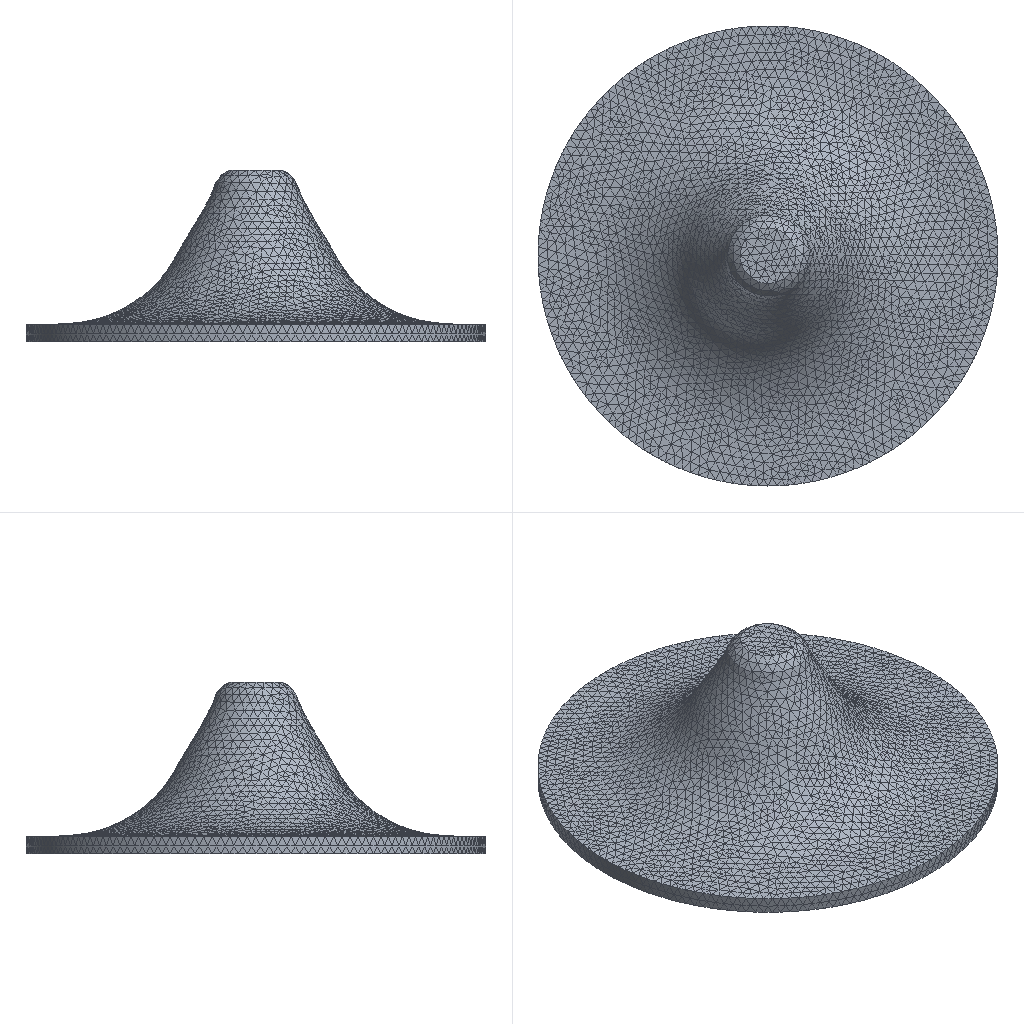Simulation study
Set-up summary:
category,name,step,type,value,unit,region
solver,ansys_mapdl
solver,version,,,22.2
units,MPA,,stated
analysis,deck,,static,static
load_step,requested,,,1
analysis,nlgeom,,,False
mesh,nodes,,,155821
mesh,elements,,,107174
element_type,ANSYS 187 (type 1),,solid,107174
load,load commands in deck,,count,1
bc,support commands in deck,,count,3
named_set,_DISPZEROUX,,component
named_set,_DISPZEROUY,,component
named_set,_DISPZEROUZ,,component
material,1,,in results
check,setup vs results,,match
Ansys APDL input file, long lists of numbers shortened:
/batch
/config,noeldb,1     ! force off writing results to database
*get,_wallstrt,active,,time,wall
! ANSYS input file written by Workbench version 2022 R2
! File used for geometry attach: D:\虚拟C盘\有限元\叶轮.x_t
/title,wbnew--____ (A5)
! ****** Begin Custom Load Command Snippet ******
/COM, ACT Extensions:
/COM,     LSDYNA, 2022.2
/COM,/COM,     ANSYSMotion, 2022.2
/COM,
! ****** End   Custom Load Command Snippet ******
*DIM,_wb_ProjectScratch_dir,string,248
_wb_ProjectScratch_dir(1) = 'C:\Users\16969\AppData\Local\Temp\WB_16969_20940_2\_ProjectScratch\Scr4E8C\'
*DIM,_wb_SolverFiles_dir,string,248
_wb_SolverFiles_dir(1) = 'C:\Users\16969\AppData\Local\Temp\WB_16969_20940_2\wbnew_files\dp0\SYS\MECH\'
*DIM,_wb_userfiles_dir,string,248
_wb_userfiles_dir(1) = 'C:\Users\16969\AppData\Local\Temp\WB_16969_20940_2\wbnew_files\user_files\'
/com,--- Data in consistent NMM units. See Solving Units in the help system for more information.
/units,MPA
/nopr
/wb,file,start              !  signify a WB generated input file
/prep7
! Turn off shape checking because checks already performed inside WB mesher.
! See help system for more information.
SHPP,OFF,,NOWARN
/nolist
etcon,set             ! allow ANSYS to choose best KEYOP's for 180x elements, resets any applicable keyopt to MAPDL defaults
/com,*********** Nodes for the whole assembly ***********
nblock,3,,171403
(1i9,3e20.9e3)
     3129     1.307338000E+02    -1.601027297E-14     1.587500000E+01
! (155820 more lines like these left out)
-1
/wb,elem,start            !  set before creation of elements
/com,*********** Elements for Body 1 "Part 17" ***********
et,1,187
eblock,19,solid,,107174
(19i9)
        1        1        1        1        0        0        0        0       10        0        1     6940    11087    24318    14385    51231    83667    51236    51233
! (214347 more lines like these left out)
-1
/wb,elem,end               !  done creating elements
/com,*********** Send User Defined Coordinate System(s) ***********
csys,0
toffst,273.15,  ! Temperature offset from absolute zero
/com,*********** Set Reference Temperature ***********
tref,22.
/wb,mat,start              !  starting to send materials
/com,*********** Send Materials ***********
Temperature = 'TEMP' ! Temperature
MP,DENS,1,2.77e-09,	! tonne mm^-3
MP,ALPX,1,2.3e-05,	! C^-1
MP,C,1,875000000,	! mm^2 s^-2 C^-1
MPTEMP,,,,,,,,
MPTEMP,1,-100
MPTEMP,2,0
MPTEMP,3,100
MPTEMP,4,200
MPDATA,KXX,1, ,114,144,165,175,	! tonne mm s^-3 C^-1
MPTEMP,,,,,,,,
MPTEMP,,,,,,,,
MPTEMP,1,0
MPTEMP,2,20
MPTEMP,3,100
MPDATA,RSVX,1, ,2.43e-05,2.67e-05,3.63e-05,	! ohm mm
MPTEMP,,,,,,,,
MP,EX,1,75000,	! tonne s^-2 mm^-1
MP,NUXY,1,0.25,
MP,MURX,1,1,
/wb,mat,end                !  done sending materials
!************************* Model Summary ********************
!Part 17,	铝合金,	matid,	1
!************************* End Model Summary ********************
! get the diagonal of the bounding box. Needed later for other things
*get,_xmin,node,,mnloc,x
*get,_ymin,node,,mnloc,y
*get,_zmin,node,,mnloc,z
*get,_xmax,node,,mxloc,x
*get,_ymax,node,,mxloc,y
*get,_zmax,node,,mxloc,z
_ASMDIAG=(_xmax-_xmin)*(_xmax-_xmin)+(_ymax-_ymin)*(_ymax-_ymin)+(_zmax-_zmin)*(_zmax-_zmin)
_ASMDIAG=SQRT(_ASMDIAG)
/wb,contact,start          !  starting to send contact
/wb,contact,end            !  done creating contacts
/golist
/wb,load,start             !  starting to send loads
/com,******* Constant Zero Displacement X *******
CMBLOCK,_DISPZEROUX,NODE,     2266
(8i10)
      3349      3350      3351      3352      3353      3354      3355      3356
! (283 more lines like these left out)
cmsel,s,_DISPZEROUX
d,all,ux,0
nsel,all
/com,******* Constant Zero Displacement Y *******
CMBLOCK,_DISPZEROUY,NODE,     2266
(8i10)
      3349      3350      3351      3352      3353      3354      3355      3356
! (283 more lines like these left out)
cmsel,s,_DISPZEROUY
d,all,uy,0
nsel,all
/com,******* Constant Zero Displacement Z *******
CMBLOCK,_DISPZEROUZ,NODE,     2266
(8i10)
      3349      3350      3351      3352      3353      3354      3355      3356
! (283 more lines like these left out)
cmsel,s,_DISPZEROUZ
d,all,uz,0
nsel,all
/com,*********** Define Rotational Velocity ***********
cglo,0.,0.,40.005
/gst,on,on
fini
*get,_numnode,node,0,count
*get,_numelem,elem,0,count
*get, _MAXELEMNUM, elem, 0, NUM, MAX
*get, _MAXNODENUM, node, 0, NUM, MAX
*get, _MAXELEMTYPE, etyp, 0, NUM, MAX
*get, _MAXREALCONST, rcon, 0, NUM, MAX
/go
/wb,load,end               !  done creating loads
/com,--- Number of total nodes = %_numnode%
/com,--- Number of contact elements = 0
/com,--- Number of spring elements = 0
/com,--- Number of bearing elements = 0
/com,--- Number of solid elements = 107174
/com,--- Number of condensed parts = 0
/com,--- Number of total elements = %_numelem%
*get,_wallbsol,active,,time,wall
/com,****************************************************************************
/com,*************************    SOLUTION       ********************************
/com,****************************************************************************
/solu
antype,0                   ! static analysis
_thickRatio=  1     ! Ratio of thick parts in the model
eqsl,pcg,1e-8,,,,,,1
cntr,print,1               ! print out contact info and also make no initial contact an error
dmpoption,emat,no             ! Don't combine emat file for DANSYS
dmpoption,esav,no             ! Don't combine esav file for DANSYS
nldiag,cont,iter           ! print out contact info each equilibrium iteration
rescontrol,,none                 ! Do not keep any restart files
/com,****************************************************
/com,******************* SOLVE FOR LS 1 OF 1 ****************
cgom,0.,0.,200.
/nopr
/gopr
nsub,1,1,1
time,1.
outres,erase
outres,all,none
outres,nsol,all,
outres,rsol,all
outres,eangl,all
outres,etmp,all
outres,veng,all
outres,strs,all,
outres,epel,all,
outres,eppl,all,
outres,cont,all,
! *********** WB SOLVE COMMAND ***********
! check interactive state
*get,ANSINTER_,active,,int
*if,ANSINTER_,ne,0,then
/eof
*endif
solve
/com *************** Write FE CONNECTORS *********
CEWRITE,file,ce,,INTE
/com,****************************************************
/com,*************** FINISHED SOLVE FOR LS 1 *************
*get,_wallasol,active,,time,wall
/nopr
*get,_numnode,node,0,count
*get,_numelem,elem,0,count
*get, _MAXELEMNUM, elem, 0, NUM, MAX
*get, _MAXNODENUM, node, 0, NUM, MAX,,,INTERNAL
*get, _MAXELEMTYPE, etyp, 0, NUM, MAX
*get, _MAXREALCONST, rcon, 0, NUM, MAX
*get,_NSOLTHREADS,active,0,ntfs
*get,_NSOLPROCESSES,active,0,npfs
/gopr
*get,_PCGITER,active,,solu,cgiter
/post1
xmlo,ENCODING,ISO-8859-1
xmlo,parm
/xml,parm,xml
fini
/gopr
*get,_walldone,active,,time,wall
_preptime=(_wallbsol-_wallstrt)*3600
_solvtime=(_wallasol-_wallbsol)*3600
_posttime=(_walldone-_wallasol)*3600
_totaltim=(_walldone-_wallstrt)*3600
*get,_dlbratio,active,0,solu,dlbr
*get,_combtime,active,0,solu,comb
*get,_ssmode,active,0,solu,ssmm
*get,_ndofs,active,0,solu,ndof
*get,_sol_end_time,active,0,set,time
*if,_sol_end_time,eq,1.,then
/fclean				!clean distributed files
*endif
/com,--- Total number of nodes = %_numnode%
/com,--- Total number of elements = %_numelem%
/com,--- Element load balance ratio = %_dlbratio%
/com,--- Time to combine distributed files = %_combtime%
/com,--- Sparse memory mode = %_ssmode%
/com,--- Number of DOF = %_ndofs%
/wb,file,end               ! done with WB generated input
Results summary:
result,analysis,,,static
result,last_loadstep,,,1
result,primary field,,,displacement
result,reaction total,1,FX,0.000116,N
result,reaction total,1,FY,-0.000871,N
result,reaction total,1,FZ,0.0,N
result,mass,,,0.003282,"NMM: mm, ton, N, s, mV, mA, degC"